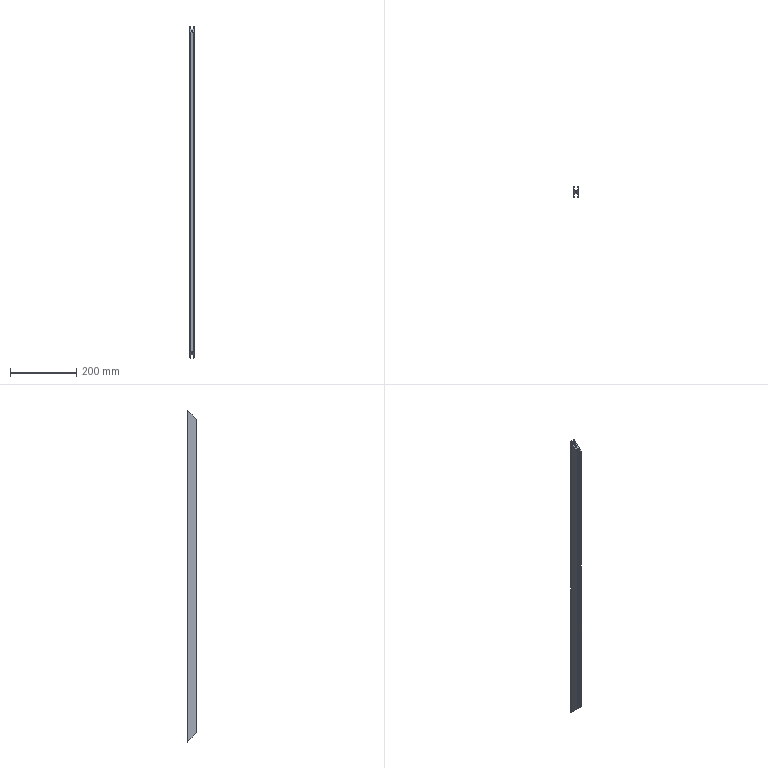Part | STEP file | OB1530-1000 | 1 solid | 36 faces | box 15 x 30 x 1000 mm | volume 237102 mm3 | plane 30 | cylinder 6 | commonest cylinder face diameters 3 x4 5 x2
STEP:
#1=CARTESIAN_POINT('',(2.5,0.,985.));
#2=VERTEX_POINT('',#1);
#3=CARTESIAN_POINT('',(-2.5,0.,985.));
#4=VERTEX_POINT('',#3);
#5=CARTESIAN_POINT('',(2.5,0.,985.));
#6=CARTESIAN_POINT('',(2.5,-5.,980.));
#7=CARTESIAN_POINT('',(-2.5,-5.,980.));
#8=CARTESIAN_POINT('',(-2.5,0.,985.));
#9=(BOUNDED_CURVE()B_SPLINE_CURVE(3,(#5,#6,#7,#8),.UNSPECIFIED.,.F.,.F.)B_SPLINE_CURVE_WITH_KNOTS((4,4),(4.712,7.854),.UNSPECIFIED.)CURVE()GEOMETRIC_REPRESENTATION_ITEM()RATIONAL_B_SPLINE_CURVE((1.,0.3333,0.3333,1.))REPRESENTATION_ITEM(''));
#10=EDGE_CURVE('',#2,#4,#9,.T.);
#11=ORIENTED_EDGE('',*,*,#10,.F.);
#12=CARTESIAN_POINT('',(2.5,0.,15.));
#13=VERTEX_POINT('',#12);
#14=CARTESIAN_POINT('',(2.5,0.,1000.));
#15=DIRECTION('',(0.,0.,-1.));
#16=VECTOR('',#15,1000.);
#17=LINE('',#14,#16);
#18=EDGE_CURVE('',#2,#13,#17,.T.);
#19=ORIENTED_EDGE('',*,*,#18,.T.);
#20=CARTESIAN_POINT('',(-2.5,0.,15.));
#21=VERTEX_POINT('',#20);
#22=CARTESIAN_POINT('',(-2.5,0.,15.));
#23=CARTESIAN_POINT('',(-2.5,-5.,20.));
#24=CARTESIAN_POINT('',(2.5,-5.,20.));
#25=CARTESIAN_POINT('',(2.5,0.,15.));
#26=(BOUNDED_CURVE()B_SPLINE_CURVE(3,(#22,#23,#24,#25),.UNSPECIFIED.,.F.,.F.)B_SPLINE_CURVE_WITH_KNOTS((4,4),(1.571,4.712),.UNSPECIFIED.)CURVE()GEOMETRIC_REPRESENTATION_ITEM()RATIONAL_B_SPLINE_CURVE((1.,0.3333,0.3333,1.))REPRESENTATION_ITEM(''));
#27=EDGE_CURVE('',#21,#13,#26,.T.);
#28=ORIENTED_EDGE('',*,*,#27,.F.);
#29=CARTESIAN_POINT('',(-2.5,0.,1000.));
#30=DIRECTION('',(0.,0.,-1.));
#31=VECTOR('',#30,1000.);
#32=LINE('',#29,#31);
#33=EDGE_CURVE('',#4,#21,#32,.T.);
#34=ORIENTED_EDGE('',*,*,#33,.F.);
#35=EDGE_LOOP('',(#11,#19,#28,#34));
#36=FACE_OUTER_BOUND('',#35,.T.);
#37=CARTESIAN_POINT('',(0.,0.,1000.));
#38=DIRECTION('',(0.,0.,-1.));
#39=DIRECTION('',(-1.,0.,0.));
#40=AXIS2_PLACEMENT_3D('',#37,#38,#39);
#41=CYLINDRICAL_SURFACE('',#40,2.5);
#42=ADVANCED_FACE('',(#36),#41,.F.);
#43=CARTESIAN_POINT('',(6.,15.,1000.));
#44=VERTEX_POINT('',#43);
#45=CARTESIAN_POINT('',(6.,15.,0.));
#46=VERTEX_POINT('',#45);
#47=CARTESIAN_POINT('',(6.,15.,1000.));
#48=DIRECTION('',(0.,0.,-1.));
#49=VECTOR('',#48,1000.);
#50=LINE('',#47,#49);
#51=EDGE_CURVE('',#44,#46,#50,.T.);
#52=ORIENTED_EDGE('',*,*,#51,.F.);
#53=CARTESIAN_POINT('',(7.5,13.5,998.5));
#54=VERTEX_POINT('',#53);
#55=CARTESIAN_POINT('',(6.,15.,1000.));
#56=CARTESIAN_POINT('',(6.879,15.,1000.));
#57=CARTESIAN_POINT('',(7.5,14.379,999.379));
#58=CARTESIAN_POINT('',(7.5,13.5,998.5));
#59=(BOUNDED_CURVE()B_SPLINE_CURVE(3,(#55,#56,#57,#58),.UNSPECIFIED.,.F.,.F.)B_SPLINE_CURVE_WITH_KNOTS((4,4),(3.142,4.712),.UNSPECIFIED.)CURVE()GEOMETRIC_REPRESENTATION_ITEM()RATIONAL_B_SPLINE_CURVE((1.,0.8047,0.8047,1.))REPRESENTATION_ITEM(''));
#60=EDGE_CURVE('',#44,#54,#59,.T.);
#61=ORIENTED_EDGE('',*,*,#60,.T.);
#62=CARTESIAN_POINT('',(7.5,13.5,1.5));
#63=VERTEX_POINT('',#62);
#64=CARTESIAN_POINT('',(7.5,13.5,1000.));
#65=DIRECTION('',(0.,0.,-1.));
#66=VECTOR('',#65,1000.);
#67=LINE('',#64,#66);
#68=EDGE_CURVE('',#54,#63,#67,.T.);
#69=ORIENTED_EDGE('',*,*,#68,.T.);
#70=CARTESIAN_POINT('',(7.5,13.5,1.5));
#71=CARTESIAN_POINT('',(7.5,14.379,0.6213));
#72=CARTESIAN_POINT('',(6.879,15.,0.));
#73=CARTESIAN_POINT('',(6.,15.,0.));
#74=(BOUNDED_CURVE()B_SPLINE_CURVE(3,(#70,#71,#72,#73),.UNSPECIFIED.,.F.,.T.)B_SPLINE_CURVE_WITH_KNOTS((4,4),(4.712,6.283),.UNSPECIFIED.)CURVE()GEOMETRIC_REPRESENTATION_ITEM()RATIONAL_B_SPLINE_CURVE((1.,0.8047,0.8047,1.))REPRESENTATION_ITEM(''));
#75=EDGE_CURVE('',#63,#46,#74,.T.);
#76=ORIENTED_EDGE('',*,*,#75,.T.);
#77=EDGE_LOOP('',(#52,#61,#69,#76));
#78=FACE_OUTER_BOUND('',#77,.T.);
#79=CARTESIAN_POINT('',(6.,13.5,1000.));
#80=DIRECTION('',(0.,0.,-1.));
#81=DIRECTION('',(-1.,0.,0.));
#82=AXIS2_PLACEMENT_3D('',#79,#80,#81);
#83=CYLINDRICAL_SURFACE('',#82,1.5);
#84=ADVANCED_FACE('',(#78),#83,.T.);
#85=CARTESIAN_POINT('',(3.25,15.,0.));
#86=VERTEX_POINT('',#85);
#87=CARTESIAN_POINT('',(6.,15.,0.));
#88=DIRECTION('',(-1.,0.,0.));
#89=VECTOR('',#88,1000.);
#90=LINE('',#87,#89);
#91=EDGE_CURVE('',#46,#86,#90,.T.);
#92=ORIENTED_EDGE('',*,*,#91,.T.);
#93=CARTESIAN_POINT('',(3.25,15.,1000.));
#94=VERTEX_POINT('',#93);
#95=CARTESIAN_POINT('',(3.25,15.,1000.));
#96=DIRECTION('',(0.,0.,-1.));
#97=VECTOR('',#96,1000.);
#98=LINE('',#95,#97);
#99=EDGE_CURVE('',#94,#86,#98,.T.);
#100=ORIENTED_EDGE('',*,*,#99,.F.);
#101=CARTESIAN_POINT('',(6.,15.,1000.));
#102=DIRECTION('',(-1.,0.,0.));
#103=VECTOR('',#102,1000.);
#104=LINE('',#101,#103);
#105=EDGE_CURVE('',#44,#94,#104,.T.);
#106=ORIENTED_EDGE('',*,*,#105,.F.);
#107=ORIENTED_EDGE('',*,*,#51,.T.);
#108=EDGE_LOOP('',(#92,#100,#106,#107));
#109=FACE_OUTER_BOUND('',#108,.T.);
#110=CARTESIAN_POINT('',(6.,15.,1000.));
#111=DIRECTION('',(0.,-1.,0.));
#112=DIRECTION('',(0.,0.,-1.));
#113=AXIS2_PLACEMENT_3D('',#110,#111,#112);
#114=PLANE('',#113);
#115=ADVANCED_FACE('',(#109),#114,.F.);
#116=CARTESIAN_POINT('',(3.25,13.,998.));
#117=VERTEX_POINT('',#116);
#118=CARTESIAN_POINT('',(3.25,13.,2.));
#119=VERTEX_POINT('',#118);
#120=CARTESIAN_POINT('',(3.25,13.,1000.));
#121=DIRECTION('',(0.,0.,-1.));
#122=VECTOR('',#121,1000.);
#123=LINE('',#120,#122);
#124=EDGE_CURVE('',#117,#119,#123,.T.);
#125=ORIENTED_EDGE('',*,*,#124,.F.);
#126=CARTESIAN_POINT('',(3.25,15.,1000.));
#127=DIRECTION('',(0.,0.7071,0.7071));
#128=VECTOR('',#127,1000.);
#129=LINE('',#126,#128);
#130=EDGE_CURVE('',#117,#94,#129,.T.);
#131=ORIENTED_EDGE('',*,*,#130,.T.);
#132=ORIENTED_EDGE('',*,*,#99,.T.);
#133=CARTESIAN_POINT('',(3.25,-485.,500.));
#134=DIRECTION('',(0.,-0.7071,0.7071));
#135=VECTOR('',#134,1000.);
#136=LINE('',#133,#135);
#137=EDGE_CURVE('',#86,#119,#136,.T.);
#138=ORIENTED_EDGE('',*,*,#137,.T.);
#139=EDGE_LOOP('',(#125,#131,#132,#138));
#140=FACE_OUTER_BOUND('',#139,.T.);
#141=CARTESIAN_POINT('',(3.25,15.,1000.));
#142=DIRECTION('',(1.,0.,0.));
#143=DIRECTION('',(0.,0.,-1.));
#144=AXIS2_PLACEMENT_3D('',#141,#142,#143);
#145=PLANE('',#144);
#146=ADVANCED_FACE('',(#140),#145,.F.);
#147=CARTESIAN_POINT('',(5.5,13.,998.));
#148=VERTEX_POINT('',#147);
#149=CARTESIAN_POINT('',(5.5,13.,2.));
#150=VERTEX_POINT('',#149);
#151=CARTESIAN_POINT('',(5.5,13.,1000.));
#152=DIRECTION('',(0.,0.,-1.));
#153=VECTOR('',#152,1000.);
#154=LINE('',#151,#153);
#155=EDGE_CURVE('',#148,#150,#154,.T.);
#156=ORIENTED_EDGE('',*,*,#155,.F.);
#157=CARTESIAN_POINT('',(3.25,13.,998.));
#158=DIRECTION('',(-1.,0.,0.));
#159=VECTOR('',#158,1000.);
#160=LINE('',#157,#159);
#161=EDGE_CURVE('',#148,#117,#160,.T.);
#162=ORIENTED_EDGE('',*,*,#161,.T.);
#163=ORIENTED_EDGE('',*,*,#124,.T.);
#164=CARTESIAN_POINT('',(3.25,13.,2.));
#165=DIRECTION('',(1.,0.,0.));
#166=VECTOR('',#165,1000.);
#167=LINE('',#164,#166);
#168=EDGE_CURVE('',#119,#150,#167,.T.);
#169=ORIENTED_EDGE('',*,*,#168,.T.);
#170=EDGE_LOOP('',(#156,#162,#163,#169));
#171=FACE_OUTER_BOUND('',#170,.T.);
#172=CARTESIAN_POINT('',(3.25,13.,1000.));
#173=DIRECTION('',(0.,1.,0.));
#174=DIRECTION('',(0.,0.,1.));
#175=AXIS2_PLACEMENT_3D('',#172,#173,#174);
#176=PLANE('',#175);
#177=ADVANCED_FACE('',(#171),#176,.F.);
#178=CARTESIAN_POINT('',(5.5,7.,992.));
#179=VERTEX_POINT('',#178);
#180=CARTESIAN_POINT('',(5.5,7.,8.));
#181=VERTEX_POINT('',#180);
#182=CARTESIAN_POINT('',(5.5,7.,1000.));
#183=DIRECTION('',(0.,0.,-1.));
#184=VECTOR('',#183,1000.);
#185=LINE('',#182,#184);
#186=EDGE_CURVE('',#179,#181,#185,.T.);
#187=ORIENTED_EDGE('',*,*,#186,.F.);
#188=CARTESIAN_POINT('',(5.5,14.,999.));
#189=DIRECTION('',(0.,0.7071,0.7071));
#190=VECTOR('',#189,1000.);
#191=LINE('',#188,#190);
#192=EDGE_CURVE('',#179,#148,#191,.T.);
#193=ORIENTED_EDGE('',*,*,#192,.T.);
#194=ORIENTED_EDGE('',*,*,#155,.T.);
#195=CARTESIAN_POINT('',(5.5,-486.,501.));
#196=DIRECTION('',(0.,-0.7071,0.7071));
#197=VECTOR('',#196,1000.);
#198=LINE('',#195,#197);
#199=EDGE_CURVE('',#150,#181,#198,.T.);
#200=ORIENTED_EDGE('',*,*,#199,.T.);
#201=EDGE_LOOP('',(#187,#193,#194,#200));
#202=FACE_OUTER_BOUND('',#201,.T.);
#203=CARTESIAN_POINT('',(5.5,13.,1000.));
#204=DIRECTION('',(1.,0.,0.));
#205=DIRECTION('',(0.,1.,0.));
#206=AXIS2_PLACEMENT_3D('',#203,#204,#205);
#207=PLANE('',#206);
#208=ADVANCED_FACE('',(#202),#207,.F.);
#209=CARTESIAN_POINT('',(3.25,7.,992.));
#210=VERTEX_POINT('',#209);
#211=CARTESIAN_POINT('',(3.25,7.,8.));
#212=VERTEX_POINT('',#211);
#213=CARTESIAN_POINT('',(3.25,7.,1000.));
#214=DIRECTION('',(0.,0.,-1.));
#215=VECTOR('',#214,1000.);
#216=LINE('',#213,#215);
#217=EDGE_CURVE('',#210,#212,#216,.T.);
#218=ORIENTED_EDGE('',*,*,#217,.F.);
#219=CARTESIAN_POINT('',(5.5,7.,992.));
#220=DIRECTION('',(1.,0.,0.));
#221=VECTOR('',#220,1000.);
#222=LINE('',#219,#221);
#223=EDGE_CURVE('',#210,#179,#222,.T.);
#224=ORIENTED_EDGE('',*,*,#223,.T.);
#225=ORIENTED_EDGE('',*,*,#186,.T.);
#226=CARTESIAN_POINT('',(5.5,7.,8.));
#227=DIRECTION('',(-1.,0.,0.));
#228=VECTOR('',#227,1000.);
#229=LINE('',#226,#228);
#230=EDGE_CURVE('',#181,#212,#229,.T.);
#231=ORIENTED_EDGE('',*,*,#230,.T.);
#232=EDGE_LOOP('',(#218,#224,#225,#231));
#233=FACE_OUTER_BOUND('',#232,.T.);
#234=CARTESIAN_POINT('',(5.5,7.,1000.));
#235=DIRECTION('',(0.,-1.,0.));
#236=DIRECTION('',(1.,0.,0.));
#237=AXIS2_PLACEMENT_3D('',#234,#235,#236);
#238=PLANE('',#237);
#239=ADVANCED_FACE('',(#233),#238,.F.);
#240=CARTESIAN_POINT('',(3.25,5.,990.));
#241=VERTEX_POINT('',#240);
#242=CARTESIAN_POINT('',(3.25,5.,10.));
#243=VERTEX_POINT('',#242);
#244=CARTESIAN_POINT('',(3.25,5.,1000.));
#245=DIRECTION('',(0.,0.,-1.));
#246=VECTOR('',#245,1000.);
#247=LINE('',#244,#246);
#248=EDGE_CURVE('',#241,#243,#247,.T.);
#249=ORIENTED_EDGE('',*,*,#248,.F.);
#250=CARTESIAN_POINT('',(3.25,11.,996.));
#251=DIRECTION('',(0.,0.7071,0.7071));
#252=VECTOR('',#251,1000.);
#253=LINE('',#250,#252);
#254=EDGE_CURVE('',#241,#210,#253,.T.);
#255=ORIENTED_EDGE('',*,*,#254,.T.);
#256=ORIENTED_EDGE('',*,*,#217,.T.);
#257=CARTESIAN_POINT('',(3.25,-489.,504.));
#258=DIRECTION('',(0.,-0.7071,0.7071));
#259=VECTOR('',#258,1000.);
#260=LINE('',#257,#259);
#261=EDGE_CURVE('',#212,#243,#260,.T.);
#262=ORIENTED_EDGE('',*,*,#261,.T.);
#263=EDGE_LOOP('',(#249,#255,#256,#262));
#264=FACE_OUTER_BOUND('',#263,.T.);
#265=CARTESIAN_POINT('',(3.25,7.,1000.));
#266=DIRECTION('',(1.,0.,0.));
#267=DIRECTION('',(0.,1.,0.));
#268=AXIS2_PLACEMENT_3D('',#265,#266,#267);
#269=PLANE('',#268);
#270=ADVANCED_FACE('',(#264),#269,.F.);
#271=CARTESIAN_POINT('',(-3.25,5.,990.));
#272=VERTEX_POINT('',#271);
#273=CARTESIAN_POINT('',(-3.25,5.,10.));
#274=VERTEX_POINT('',#273);
#275=CARTESIAN_POINT('',(-3.25,5.,1000.));
#276=DIRECTION('',(0.,0.,-1.));
#277=VECTOR('',#276,1000.);
#278=LINE('',#275,#277);
#279=EDGE_CURVE('',#272,#274,#278,.T.);
#280=ORIENTED_EDGE('',*,*,#279,.F.);
#281=CARTESIAN_POINT('',(3.25,5.,990.));
#282=DIRECTION('',(1.,0.,0.));
#283=VECTOR('',#282,1000.);
#284=LINE('',#281,#283);
#285=EDGE_CURVE('',#272,#241,#284,.T.);
#286=ORIENTED_EDGE('',*,*,#285,.T.);
#287=ORIENTED_EDGE('',*,*,#248,.T.);
#288=CARTESIAN_POINT('',(3.25,5.,10.));
#289=DIRECTION('',(-1.,0.,0.));
#290=VECTOR('',#289,1000.);
#291=LINE('',#288,#290);
#292=EDGE_CURVE('',#243,#274,#291,.T.);
#293=ORIENTED_EDGE('',*,*,#292,.T.);
#294=EDGE_LOOP('',(#280,#286,#287,#293));
#295=FACE_OUTER_BOUND('',#294,.T.);
#296=CARTESIAN_POINT('',(3.25,5.,1000.));
#297=DIRECTION('',(0.,-1.,0.));
#298=DIRECTION('',(0.,0.,-1.));
#299=AXIS2_PLACEMENT_3D('',#296,#297,#298);
#300=PLANE('',#299);
#301=ADVANCED_FACE('',(#295),#300,.F.);
#302=CARTESIAN_POINT('',(-3.25,7.,992.));
#303=VERTEX_POINT('',#302);
#304=CARTESIAN_POINT('',(-3.25,7.,8.));
#305=VERTEX_POINT('',#304);
#306=CARTESIAN_POINT('',(-3.25,7.,1000.));
#307=DIRECTION('',(0.,0.,-1.));
#308=VECTOR('',#307,1000.);
#309=LINE('',#306,#308);
#310=EDGE_CURVE('',#303,#305,#309,.T.);
#311=ORIENTED_EDGE('',*,*,#310,.F.);
#312=CARTESIAN_POINT('',(-3.25,11.,996.));
#313=DIRECTION('',(0.,-0.7071,-0.7071));
#314=VECTOR('',#313,1000.);
#315=LINE('',#312,#314);
#316=EDGE_CURVE('',#303,#272,#315,.T.);
#317=ORIENTED_EDGE('',*,*,#316,.T.);
#318=ORIENTED_EDGE('',*,*,#279,.T.);
#319=CARTESIAN_POINT('',(-3.25,-489.,504.));
#320=DIRECTION('',(0.,0.7071,-0.7071));
#321=VECTOR('',#320,1000.);
#322=LINE('',#319,#321);
#323=EDGE_CURVE('',#274,#305,#322,.T.);
#324=ORIENTED_EDGE('',*,*,#323,.T.);
#325=EDGE_LOOP('',(#311,#317,#318,#324));
#326=FACE_OUTER_BOUND('',#325,.T.);
#327=CARTESIAN_POINT('',(-3.25,7.,1000.));
#328=DIRECTION('',(-1.,0.,0.));
#329=DIRECTION('',(0.,-1.,0.));
#330=AXIS2_PLACEMENT_3D('',#327,#328,#329);
#331=PLANE('',#330);
#332=ADVANCED_FACE('',(#326),#331,.F.);
#333=CARTESIAN_POINT('',(-5.5,7.,992.));
#334=VERTEX_POINT('',#333);
#335=CARTESIAN_POINT('',(-5.5,7.,8.));
#336=VERTEX_POINT('',#335);
#337=CARTESIAN_POINT('',(-5.5,7.,1000.));
#338=DIRECTION('',(0.,0.,-1.));
#339=VECTOR('',#338,1000.);
#340=LINE('',#337,#339);
#341=EDGE_CURVE('',#334,#336,#340,.T.);
#342=ORIENTED_EDGE('',*,*,#341,.F.);
#343=CARTESIAN_POINT('',(-5.5,7.,992.));
#344=DIRECTION('',(1.,0.,0.));
#345=VECTOR('',#344,1000.);
#346=LINE('',#343,#345);
#347=EDGE_CURVE('',#334,#303,#346,.T.);
#348=ORIENTED_EDGE('',*,*,#347,.T.);
#349=ORIENTED_EDGE('',*,*,#310,.T.);
#350=CARTESIAN_POINT('',(-5.5,7.,8.));
#351=DIRECTION('',(-1.,0.,0.));
#352=VECTOR('',#351,1000.);
#353=LINE('',#350,#352);
#354=EDGE_CURVE('',#305,#336,#353,.T.);
#355=ORIENTED_EDGE('',*,*,#354,.T.);
#356=EDGE_LOOP('',(#342,#348,#349,#355));
#357=FACE_OUTER_BOUND('',#356,.T.);
#358=CARTESIAN_POINT('',(-5.5,7.,1000.));
#359=DIRECTION('',(0.,-1.,0.));
#360=DIRECTION('',(1.,0.,0.));
#361=AXIS2_PLACEMENT_3D('',#358,#359,#360);
#362=PLANE('',#361);
#363=ADVANCED_FACE('',(#357),#362,.F.);
#364=CARTESIAN_POINT('',(-5.5,13.,998.));
#365=VERTEX_POINT('',#364);
#366=CARTESIAN_POINT('',(-5.5,13.,2.));
#367=VERTEX_POINT('',#366);
#368=CARTESIAN_POINT('',(-5.5,13.,1000.));
#369=DIRECTION('',(0.,0.,-1.));
#370=VECTOR('',#369,1000.);
#371=LINE('',#368,#370);
#372=EDGE_CURVE('',#365,#367,#371,.T.);
#373=ORIENTED_EDGE('',*,*,#372,.F.);
#374=CARTESIAN_POINT('',(-5.5,14.,999.));
#375=DIRECTION('',(0.,-0.7071,-0.7071));
#376=VECTOR('',#375,1000.);
#377=LINE('',#374,#376);
#378=EDGE_CURVE('',#365,#334,#377,.T.);
#379=ORIENTED_EDGE('',*,*,#378,.T.);
#380=ORIENTED_EDGE('',*,*,#341,.T.);
#381=CARTESIAN_POINT('',(-5.5,-486.,501.));
#382=DIRECTION('',(0.,0.7071,-0.7071));
#383=VECTOR('',#382,1000.);
#384=LINE('',#381,#383);
#385=EDGE_CURVE('',#336,#367,#384,.T.);
#386=ORIENTED_EDGE('',*,*,#385,.T.);
#387=EDGE_LOOP('',(#373,#379,#380,#386));
#388=FACE_OUTER_BOUND('',#387,.T.);
#389=CARTESIAN_POINT('',(-5.5,13.,1000.));
#390=DIRECTION('',(-1.,0.,0.));
#391=DIRECTION('',(0.,-1.,0.));
#392=AXIS2_PLACEMENT_3D('',#389,#390,#391);
#393=PLANE('',#392);
#394=ADVANCED_FACE('',(#388),#393,.F.);
#395=CARTESIAN_POINT('',(-3.25,13.,998.));
#396=VERTEX_POINT('',#395);
#397=CARTESIAN_POINT('',(-3.25,13.,2.));
#398=VERTEX_POINT('',#397);
#399=CARTESIAN_POINT('',(-3.25,13.,1000.));
#400=DIRECTION('',(0.,0.,-1.));
#401=VECTOR('',#400,1000.);
#402=LINE('',#399,#401);
#403=EDGE_CURVE('',#396,#398,#402,.T.);
#404=ORIENTED_EDGE('',*,*,#403,.F.);
#405=CARTESIAN_POINT('',(-3.25,13.,998.));
#406=DIRECTION('',(-1.,0.,0.));
#407=VECTOR('',#406,1000.);
#408=LINE('',#405,#407);
#409=EDGE_CURVE('',#396,#365,#408,.T.);
#410=ORIENTED_EDGE('',*,*,#409,.T.);
#411=ORIENTED_EDGE('',*,*,#372,.T.);
#412=CARTESIAN_POINT('',(-3.25,13.,2.));
#413=DIRECTION('',(1.,0.,0.));
#414=VECTOR('',#413,1000.);
#415=LINE('',#412,#414);
#416=EDGE_CURVE('',#367,#398,#415,.T.);
#417=ORIENTED_EDGE('',*,*,#416,.T.);
#418=EDGE_LOOP('',(#404,#410,#411,#417));
#419=FACE_OUTER_BOUND('',#418,.T.);
#420=CARTESIAN_POINT('',(-3.25,13.,1000.));
#421=DIRECTION('',(0.,1.,0.));
#422=DIRECTION('',(0.,0.,1.));
#423=AXIS2_PLACEMENT_3D('',#420,#421,#422);
#424=PLANE('',#423);
#425=ADVANCED_FACE('',(#419),#424,.F.);
#426=CARTESIAN_POINT('',(-3.25,15.,1000.));
#427=VERTEX_POINT('',#426);
#428=CARTESIAN_POINT('',(-3.25,15.,0.));
#429=VERTEX_POINT('',#428);
#430=CARTESIAN_POINT('',(-3.25,15.,1000.));
#431=DIRECTION('',(0.,0.,-1.));
#432=VECTOR('',#431,1000.);
#433=LINE('',#430,#432);
#434=EDGE_CURVE('',#427,#429,#433,.T.);
#435=ORIENTED_EDGE('',*,*,#434,.F.);
#436=CARTESIAN_POINT('',(-3.25,15.,1000.));
#437=DIRECTION('',(0.,-0.7071,-0.7071));
#438=VECTOR('',#437,1000.);
#439=LINE('',#436,#438);
#440=EDGE_CURVE('',#427,#396,#439,.T.);
#441=ORIENTED_EDGE('',*,*,#440,.T.);
#442=ORIENTED_EDGE('',*,*,#403,.T.);
#443=CARTESIAN_POINT('',(-3.25,-485.,500.));
#444=DIRECTION('',(0.,0.7071,-0.7071));
#445=VECTOR('',#444,1000.);
#446=LINE('',#443,#445);
#447=EDGE_CURVE('',#398,#429,#446,.T.);
#448=ORIENTED_EDGE('',*,*,#447,.T.);
#449=EDGE_LOOP('',(#435,#441,#442,#448));
#450=FACE_OUTER_BOUND('',#449,.T.);
#451=CARTESIAN_POINT('',(-3.25,15.,1000.));
#452=DIRECTION('',(-1.,0.,0.));
#453=DIRECTION('',(0.,0.,1.));
#454=AXIS2_PLACEMENT_3D('',#451,#452,#453);
#455=PLANE('',#454);
#456=ADVANCED_FACE('',(#450),#455,.F.);
#457=CARTESIAN_POINT('',(-6.,15.,0.));
#458=VERTEX_POINT('',#457);
#459=CARTESIAN_POINT('',(-6.,15.,0.));
#460=DIRECTION('',(-1.,0.,0.));
#461=VECTOR('',#460,1000.);
#462=LINE('',#459,#461);
#463=EDGE_CURVE('',#429,#458,#462,.T.);
#464=ORIENTED_EDGE('',*,*,#463,.T.);
#465=CARTESIAN_POINT('',(-6.,15.,1000.));
#466=VERTEX_POINT('',#465);
#467=CARTESIAN_POINT('',(-6.,15.,1000.));
#468=DIRECTION('',(0.,0.,-1.));
#469=VECTOR('',#468,1000.);
#470=LINE('',#467,#469);
#471=EDGE_CURVE('',#466,#458,#470,.T.);
#472=ORIENTED_EDGE('',*,*,#471,.F.);
#473=CARTESIAN_POINT('',(-6.,15.,1000.));
#474=DIRECTION('',(-1.,0.,0.));
#475=VECTOR('',#474,1000.);
#476=LINE('',#473,#475);
#477=EDGE_CURVE('',#427,#466,#476,.T.);
#478=ORIENTED_EDGE('',*,*,#477,.F.);
#479=ORIENTED_EDGE('',*,*,#434,.T.);
#480=EDGE_LOOP('',(#464,#472,#478,#479));
#481=FACE_OUTER_BOUND('',#480,.T.);
#482=CARTESIAN_POINT('',(-6.,15.,1000.));
#483=DIRECTION('',(0.,-1.,0.));
#484=DIRECTION('',(0.,0.,-1.));
#485=AXIS2_PLACEMENT_3D('',#482,#483,#484);
#486=PLANE('',#485);
#487=ADVANCED_FACE('',(#481),#486,.F.);
#488=CARTESIAN_POINT('',(-7.5,13.5,998.5));
#489=VERTEX_POINT('',#488);
#490=CARTESIAN_POINT('',(-7.5,13.5,1.5));
#491=VERTEX_POINT('',#490);
#492=CARTESIAN_POINT('',(-7.5,13.5,1000.));
#493=DIRECTION('',(0.,0.,-1.));
#494=VECTOR('',#493,1000.);
#495=LINE('',#492,#494);
#496=EDGE_CURVE('',#489,#491,#495,.T.);
#497=ORIENTED_EDGE('',*,*,#496,.F.);
#498=CARTESIAN_POINT('',(-7.5,13.5,998.5));
#499=CARTESIAN_POINT('',(-7.5,14.379,999.379));
#500=CARTESIAN_POINT('',(-6.879,15.,1000.));
#501=CARTESIAN_POINT('',(-6.,15.,1000.));
#502=(BOUNDED_CURVE()B_SPLINE_CURVE(3,(#498,#499,#500,#501),.UNSPECIFIED.,.F.,.F.)B_SPLINE_CURVE_WITH_KNOTS((4,4),(1.571,3.142),.UNSPECIFIED.)CURVE()GEOMETRIC_REPRESENTATION_ITEM()RATIONAL_B_SPLINE_CURVE((1.,0.8047,0.8047,1.))REPRESENTATION_ITEM(''));
#503=EDGE_CURVE('',#489,#466,#502,.T.);
#504=ORIENTED_EDGE('',*,*,#503,.T.);
#505=ORIENTED_EDGE('',*,*,#471,.T.);
#506=CARTESIAN_POINT('',(-6.,15.,0.));
#507=CARTESIAN_POINT('',(-6.879,15.,0.));
#508=CARTESIAN_POINT('',(-7.5,14.379,0.6213));
#509=CARTESIAN_POINT('',(-7.5,13.5,1.5));
#510=(BOUNDED_CURVE()B_SPLINE_CURVE(3,(#506,#507,#508,#509),.UNSPECIFIED.,.F.,.F.)B_SPLINE_CURVE_WITH_KNOTS((4,4),(0.,1.571),.UNSPECIFIED.)CURVE()GEOMETRIC_REPRESENTATION_ITEM()RATIONAL_B_SPLINE_CURVE((1.,0.8047,0.8047,1.))REPRESENTATION_ITEM(''));
#511=EDGE_CURVE('',#458,#491,#510,.T.);
#512=ORIENTED_EDGE('',*,*,#511,.T.);
#513=EDGE_LOOP('',(#497,#504,#505,#512));
#514=FACE_OUTER_BOUND('',#513,.T.);
#515=CARTESIAN_POINT('',(-6.,13.5,1000.));
#516=DIRECTION('',(0.,0.,-1.));
#517=DIRECTION('',(-1.,0.,0.));
#518=AXIS2_PLACEMENT_3D('',#515,#516,#517);
#519=CYLINDRICAL_SURFACE('',#518,1.5);
#520=ADVANCED_FACE('',(#514),#519,.T.);
#521=CARTESIAN_POINT('',(-7.5,-13.5,971.5));
#522=VERTEX_POINT('',#521);
#523=CARTESIAN_POINT('',(-7.5,-13.5,28.5));
#524=VERTEX_POINT('',#523);
#525=CARTESIAN_POINT('',(-7.5,-13.5,1000.));
#526=DIRECTION('',(0.,0.,-1.));
#527=VECTOR('',#526,1000.);
#528=LINE('',#525,#527);
#529=EDGE_CURVE('',#522,#524,#528,.T.);
#530=ORIENTED_EDGE('',*,*,#529,.F.);
#531=CARTESIAN_POINT('',(-7.5,-15.,970.));
#532=DIRECTION('',(0.,-0.7071,-0.7071));
#533=VECTOR('',#532,1000.);
#534=LINE('',#531,#533);
#535=EDGE_CURVE('',#489,#522,#534,.T.);
#536=ORIENTED_EDGE('',*,*,#535,.F.);
#537=ORIENTED_EDGE('',*,*,#496,.T.);
#538=CARTESIAN_POINT('',(-7.5,15.,0.));
#539=DIRECTION('',(0.,0.7071,-0.7071));
#540=VECTOR('',#539,1000.);
#541=LINE('',#538,#540);
#542=EDGE_CURVE('',#524,#491,#541,.T.);
#543=ORIENTED_EDGE('',*,*,#542,.F.);
#544=EDGE_LOOP('',(#530,#536,#537,#543));
#545=FACE_OUTER_BOUND('',#544,.T.);
#546=CARTESIAN_POINT('',(-7.5,-13.5,1000.));
#547=DIRECTION('',(1.,0.,0.));
#548=DIRECTION('',(0.,0.,-1.));
#549=AXIS2_PLACEMENT_3D('',#546,#547,#548);
#550=PLANE('',#549);
#551=ADVANCED_FACE('',(#545),#550,.F.);
#552=CARTESIAN_POINT('',(-6.,-15.,970.));
#553=VERTEX_POINT('',#552);
#554=CARTESIAN_POINT('',(-6.,-15.,30.));
#555=VERTEX_POINT('',#554);
#556=CARTESIAN_POINT('',(-6.,-15.,1000.));
#557=DIRECTION('',(0.,0.,-1.));
#558=VECTOR('',#557,1000.);
#559=LINE('',#556,#558);
#560=EDGE_CURVE('',#553,#555,#559,.T.);
#561=ORIENTED_EDGE('',*,*,#560,.F.);
#562=CARTESIAN_POINT('',(-6.,-15.,970.));
#563=CARTESIAN_POINT('',(-6.879,-15.,970.));
#564=CARTESIAN_POINT('',(-7.5,-14.379,970.621));
#565=CARTESIAN_POINT('',(-7.5,-13.5,971.5));
#566=(BOUNDED_CURVE()B_SPLINE_CURVE(3,(#562,#563,#564,#565),.UNSPECIFIED.,.F.,.F.)B_SPLINE_CURVE_WITH_KNOTS((4,4),(0.,1.571),.UNSPECIFIED.)CURVE()GEOMETRIC_REPRESENTATION_ITEM()RATIONAL_B_SPLINE_CURVE((1.,0.8047,0.8047,1.))REPRESENTATION_ITEM(''));
#567=EDGE_CURVE('',#553,#522,#566,.T.);
#568=ORIENTED_EDGE('',*,*,#567,.T.);
#569=ORIENTED_EDGE('',*,*,#529,.T.);
#570=CARTESIAN_POINT('',(-7.5,-13.5,28.5));
#571=CARTESIAN_POINT('',(-7.5,-14.379,29.379));
#572=CARTESIAN_POINT('',(-6.879,-15.,30.));
#573=CARTESIAN_POINT('',(-6.,-15.,30.));
#574=(BOUNDED_CURVE()B_SPLINE_CURVE(3,(#570,#571,#572,#573),.UNSPECIFIED.,.F.,.T.)B_SPLINE_CURVE_WITH_KNOTS((4,4),(1.571,3.142),.UNSPECIFIED.)CURVE()GEOMETRIC_REPRESENTATION_ITEM()RATIONAL_B_SPLINE_CURVE((1.,0.8047,0.8047,1.))REPRESENTATION_ITEM(''));
#575=EDGE_CURVE('',#524,#555,#574,.T.);
#576=ORIENTED_EDGE('',*,*,#575,.T.);
#577=EDGE_LOOP('',(#561,#568,#569,#576));
#578=FACE_OUTER_BOUND('',#577,.T.);
#579=CARTESIAN_POINT('',(-6.,-13.5,1000.));
#580=DIRECTION('',(0.,0.,-1.));
#581=DIRECTION('',(-1.,0.,0.));
#582=AXIS2_PLACEMENT_3D('',#579,#580,#581);
#583=CYLINDRICAL_SURFACE('',#582,1.5);
#584=ADVANCED_FACE('',(#578),#583,.T.);
#585=CARTESIAN_POINT('',(-3.25,-15.,970.));
#586=VERTEX_POINT('',#585);
#587=CARTESIAN_POINT('',(-3.25,-15.,30.));
#588=VERTEX_POINT('',#587);
#589=CARTESIAN_POINT('',(-3.25,-15.,1000.));
#590=DIRECTION('',(0.,0.,-1.));
#591=VECTOR('',#590,1000.);
#592=LINE('',#589,#591);
#593=EDGE_CURVE('',#586,#588,#592,.T.);
#594=ORIENTED_EDGE('',*,*,#593,.F.);
#595=CARTESIAN_POINT('',(7.5,-15.,970.));
#596=DIRECTION('',(-1.,0.,0.));
#597=VECTOR('',#596,1000.);
#598=LINE('',#595,#597);
#599=EDGE_CURVE('',#586,#553,#598,.T.);
#600=ORIENTED_EDGE('',*,*,#599,.T.);
#601=ORIENTED_EDGE('',*,*,#560,.T.);
#602=CARTESIAN_POINT('',(7.5,-15.,30.));
#603=DIRECTION('',(-1.,0.,0.));
#604=VECTOR('',#603,1000.);
#605=LINE('',#602,#604);
#606=EDGE_CURVE('',#588,#555,#605,.T.);
#607=ORIENTED_EDGE('',*,*,#606,.F.);
#608=EDGE_LOOP('',(#594,#600,#601,#607));
#609=FACE_OUTER_BOUND('',#608,.T.);
#610=CARTESIAN_POINT('',(-6.,-15.,1000.));
#611=DIRECTION('',(0.,1.,0.));
#612=DIRECTION('',(0.,0.,1.));
#613=AXIS2_PLACEMENT_3D('',#610,#611,#612);
#614=PLANE('',#613);
#615=ADVANCED_FACE('',(#609),#614,.F.);
#616=CARTESIAN_POINT('',(-3.25,-13.,972.));
#617=VERTEX_POINT('',#616);
#618=CARTESIAN_POINT('',(-3.25,-13.,28.));
#619=VERTEX_POINT('',#618);
#620=CARTESIAN_POINT('',(-3.25,-13.,1000.));
#621=DIRECTION('',(0.,0.,-1.));
#622=VECTOR('',#621,1000.);
#623=LINE('',#620,#622);
#624=EDGE_CURVE('',#617,#619,#623,.T.);
#625=ORIENTED_EDGE('',*,*,#624,.F.);
#626=CARTESIAN_POINT('',(-3.25,0.,985.));
#627=DIRECTION('',(0.,-0.7071,-0.7071));
#628=VECTOR('',#627,1000.);
#629=LINE('',#626,#628);
#630=EDGE_CURVE('',#617,#586,#629,.T.);
#631=ORIENTED_EDGE('',*,*,#630,.T.);
#632=ORIENTED_EDGE('',*,*,#593,.T.);
#633=CARTESIAN_POINT('',(-3.25,-500.,515.));
#634=DIRECTION('',(0.,0.7071,-0.7071));
#635=VECTOR('',#634,1000.);
#636=LINE('',#633,#635);
#637=EDGE_CURVE('',#588,#619,#636,.T.);
#638=ORIENTED_EDGE('',*,*,#637,.T.);
#639=EDGE_LOOP('',(#625,#631,#632,#638));
#640=FACE_OUTER_BOUND('',#639,.T.);
#641=CARTESIAN_POINT('',(-3.25,-15.,1000.));
#642=DIRECTION('',(-1.,0.,0.));
#643=DIRECTION('',(0.,0.,1.));
#644=AXIS2_PLACEMENT_3D('',#641,#642,#643);
#645=PLANE('',#644);
#646=ADVANCED_FACE('',(#640),#645,.F.);
#647=CARTESIAN_POINT('',(-5.5,-13.,972.));
#648=VERTEX_POINT('',#647);
#649=CARTESIAN_POINT('',(-5.5,-13.,28.));
#650=VERTEX_POINT('',#649);
#651=CARTESIAN_POINT('',(-5.5,-13.,1000.));
#652=DIRECTION('',(0.,0.,-1.));
#653=VECTOR('',#652,1000.);
#654=LINE('',#651,#653);
#655=EDGE_CURVE('',#648,#650,#654,.T.);
#656=ORIENTED_EDGE('',*,*,#655,.F.);
#657=CARTESIAN_POINT('',(-3.25,-13.,972.));
#658=DIRECTION('',(1.,0.,0.));
#659=VECTOR('',#658,1000.);
#660=LINE('',#657,#659);
#661=EDGE_CURVE('',#648,#617,#660,.T.);
#662=ORIENTED_EDGE('',*,*,#661,.T.);
#663=ORIENTED_EDGE('',*,*,#624,.T.);
#664=CARTESIAN_POINT('',(-3.25,-13.,28.));
#665=DIRECTION('',(-1.,0.,0.));
#666=VECTOR('',#665,1000.);
#667=LINE('',#664,#666);
#668=EDGE_CURVE('',#619,#650,#667,.T.);
#669=ORIENTED_EDGE('',*,*,#668,.T.);
#670=EDGE_LOOP('',(#656,#662,#663,#669));
#671=FACE_OUTER_BOUND('',#670,.T.);
#672=CARTESIAN_POINT('',(-3.25,-13.,1000.));
#673=DIRECTION('',(0.,-1.,0.));
#674=DIRECTION('',(0.,0.,-1.));
#675=AXIS2_PLACEMENT_3D('',#672,#673,#674);
#676=PLANE('',#675);
#677=ADVANCED_FACE('',(#671),#676,.F.);
#678=CARTESIAN_POINT('',(-5.5,-7.,978.));
#679=VERTEX_POINT('',#678);
#680=CARTESIAN_POINT('',(-5.5,-7.,22.));
#681=VERTEX_POINT('',#680);
#682=CARTESIAN_POINT('',(-5.5,-7.,1000.));
#683=DIRECTION('',(0.,0.,-1.));
#684=VECTOR('',#683,1000.);
#685=LINE('',#682,#684);
#686=EDGE_CURVE('',#679,#681,#685,.T.);
#687=ORIENTED_EDGE('',*,*,#686,.F.);
#688=CARTESIAN_POINT('',(-5.5,1.,986.));
#689=DIRECTION('',(0.,-0.7071,-0.7071));
#690=VECTOR('',#689,1000.);
#691=LINE('',#688,#690);
#692=EDGE_CURVE('',#679,#648,#691,.T.);
#693=ORIENTED_EDGE('',*,*,#692,.T.);
#694=ORIENTED_EDGE('',*,*,#655,.T.);
#695=CARTESIAN_POINT('',(-5.5,-499.,514.));
#696=DIRECTION('',(0.,0.7071,-0.7071));
#697=VECTOR('',#696,1000.);
#698=LINE('',#695,#697);
#699=EDGE_CURVE('',#650,#681,#698,.T.);
#700=ORIENTED_EDGE('',*,*,#699,.T.);
#701=EDGE_LOOP('',(#687,#693,#694,#700));
#702=FACE_OUTER_BOUND('',#701,.T.);
#703=CARTESIAN_POINT('',(-5.5,-13.,1000.));
#704=DIRECTION('',(-1.,0.,0.));
#705=DIRECTION('',(0.,-1.,0.));
#706=AXIS2_PLACEMENT_3D('',#703,#704,#705);
#707=PLANE('',#706);
#708=ADVANCED_FACE('',(#702),#707,.F.);
#709=CARTESIAN_POINT('',(-3.25,-7.,978.));
#710=VERTEX_POINT('',#709);
#711=CARTESIAN_POINT('',(-3.25,-7.,22.));
#712=VERTEX_POINT('',#711);
#713=CARTESIAN_POINT('',(-3.25,-7.,1000.));
#714=DIRECTION('',(0.,0.,-1.));
#715=VECTOR('',#714,1000.);
#716=LINE('',#713,#715);
#717=EDGE_CURVE('',#710,#712,#716,.T.);
#718=ORIENTED_EDGE('',*,*,#717,.F.);
#719=CARTESIAN_POINT('',(-5.5,-7.,978.));
#720=DIRECTION('',(-1.,0.,0.));
#721=VECTOR('',#720,1000.);
#722=LINE('',#719,#721);
#723=EDGE_CURVE('',#710,#679,#722,.T.);
#724=ORIENTED_EDGE('',*,*,#723,.T.);
#725=ORIENTED_EDGE('',*,*,#686,.T.);
#726=CARTESIAN_POINT('',(-5.5,-7.,22.));
#727=DIRECTION('',(1.,0.,0.));
#728=VECTOR('',#727,1000.);
#729=LINE('',#726,#728);
#730=EDGE_CURVE('',#681,#712,#729,.T.);
#731=ORIENTED_EDGE('',*,*,#730,.T.);
#732=EDGE_LOOP('',(#718,#724,#725,#731));
#733=FACE_OUTER_BOUND('',#732,.T.);
#734=CARTESIAN_POINT('',(-5.5,-7.,1000.));
#735=DIRECTION('',(0.,1.,0.));
#736=DIRECTION('',(-1.,0.,0.));
#737=AXIS2_PLACEMENT_3D('',#734,#735,#736);
#738=PLANE('',#737);
#739=ADVANCED_FACE('',(#733),#738,.F.);
#740=CARTESIAN_POINT('',(-3.25,-5.,980.));
#741=VERTEX_POINT('',#740);
#742=CARTESIAN_POINT('',(-3.25,-5.,20.));
#743=VERTEX_POINT('',#742);
#744=CARTESIAN_POINT('',(-3.25,-5.,1000.));
#745=DIRECTION('',(0.,0.,-1.));
#746=VECTOR('',#745,1000.);
#747=LINE('',#744,#746);
#748=EDGE_CURVE('',#741,#743,#747,.T.);
#749=ORIENTED_EDGE('',*,*,#748,.F.);
#750=CARTESIAN_POINT('',(-3.25,4.,989.));
#751=DIRECTION('',(0.,-0.7071,-0.7071));
#752=VECTOR('',#751,1000.);
#753=LINE('',#750,#752);
#754=EDGE_CURVE('',#741,#710,#753,.T.);
#755=ORIENTED_EDGE('',*,*,#754,.T.);
#756=ORIENTED_EDGE('',*,*,#717,.T.);
#757=CARTESIAN_POINT('',(-3.25,-496.,511.));
#758=DIRECTION('',(0.,0.7071,-0.7071));
#759=VECTOR('',#758,1000.);
#760=LINE('',#757,#759);
#761=EDGE_CURVE('',#712,#743,#760,.T.);
#762=ORIENTED_EDGE('',*,*,#761,.T.);
#763=EDGE_LOOP('',(#749,#755,#756,#762));
#764=FACE_OUTER_BOUND('',#763,.T.);
#765=CARTESIAN_POINT('',(-3.25,-7.,1000.));
#766=DIRECTION('',(-1.,0.,0.));
#767=DIRECTION('',(0.,-1.,0.));
#768=AXIS2_PLACEMENT_3D('',#765,#766,#767);
#769=PLANE('',#768);
#770=ADVANCED_FACE('',(#764),#769,.F.);
#771=CARTESIAN_POINT('',(3.25,-5.,980.));
#772=VERTEX_POINT('',#771);
#773=CARTESIAN_POINT('',(3.25,-5.,20.));
#774=VERTEX_POINT('',#773);
#775=CARTESIAN_POINT('',(3.25,-5.,1000.));
#776=DIRECTION('',(0.,0.,-1.));
#777=VECTOR('',#776,1000.);
#778=LINE('',#775,#777);
#779=EDGE_CURVE('',#772,#774,#778,.T.);
#780=ORIENTED_EDGE('',*,*,#779,.F.);
#781=CARTESIAN_POINT('',(3.25,-5.,980.));
#782=DIRECTION('',(-1.,0.,0.));
#783=VECTOR('',#782,1000.);
#784=LINE('',#781,#783);
#785=EDGE_CURVE('',#772,#741,#784,.T.);
#786=ORIENTED_EDGE('',*,*,#785,.T.);
#787=ORIENTED_EDGE('',*,*,#748,.T.);
#788=CARTESIAN_POINT('',(3.25,-5.,20.));
#789=DIRECTION('',(1.,0.,0.));
#790=VECTOR('',#789,1000.);
#791=LINE('',#788,#790);
#792=EDGE_CURVE('',#743,#774,#791,.T.);
#793=ORIENTED_EDGE('',*,*,#792,.T.);
#794=EDGE_LOOP('',(#780,#786,#787,#793));
#795=FACE_OUTER_BOUND('',#794,.T.);
#796=CARTESIAN_POINT('',(3.25,-5.,1000.));
#797=DIRECTION('',(0.,1.,0.));
#798=DIRECTION('',(0.,0.,1.));
#799=AXIS2_PLACEMENT_3D('',#796,#797,#798);
#800=PLANE('',#799);
#801=ADVANCED_FACE('',(#795),#800,.F.);
#802=CARTESIAN_POINT('',(3.25,-7.,978.));
#803=VERTEX_POINT('',#802);
#804=CARTESIAN_POINT('',(3.25,-7.,22.));
#805=VERTEX_POINT('',#804);
#806=CARTESIAN_POINT('',(3.25,-7.,1000.));
#807=DIRECTION('',(0.,0.,-1.));
#808=VECTOR('',#807,1000.);
#809=LINE('',#806,#808);
#810=EDGE_CURVE('',#803,#805,#809,.T.);
#811=ORIENTED_EDGE('',*,*,#810,.F.);
#812=CARTESIAN_POINT('',(3.25,4.,989.));
#813=DIRECTION('',(0.,0.7071,0.7071));
#814=VECTOR('',#813,1000.);
#815=LINE('',#812,#814);
#816=EDGE_CURVE('',#803,#772,#815,.T.);
#817=ORIENTED_EDGE('',*,*,#816,.T.);
#818=ORIENTED_EDGE('',*,*,#779,.T.);
#819=CARTESIAN_POINT('',(3.25,-496.,511.));
#820=DIRECTION('',(0.,-0.7071,0.7071));
#821=VECTOR('',#820,1000.);
#822=LINE('',#819,#821);
#823=EDGE_CURVE('',#774,#805,#822,.T.);
#824=ORIENTED_EDGE('',*,*,#823,.T.);
#825=EDGE_LOOP('',(#811,#817,#818,#824));
#826=FACE_OUTER_BOUND('',#825,.T.);
#827=CARTESIAN_POINT('',(3.25,-7.,1000.));
#828=DIRECTION('',(1.,0.,0.));
#829=DIRECTION('',(0.,1.,0.));
#830=AXIS2_PLACEMENT_3D('',#827,#828,#829);
#831=PLANE('',#830);
#832=ADVANCED_FACE('',(#826),#831,.F.);
#833=CARTESIAN_POINT('',(5.5,-7.,978.));
#834=VERTEX_POINT('',#833);
#835=CARTESIAN_POINT('',(5.5,-7.,22.));
#836=VERTEX_POINT('',#835);
#837=CARTESIAN_POINT('',(5.5,-7.,1000.));
#838=DIRECTION('',(0.,0.,-1.));
#839=VECTOR('',#838,1000.);
#840=LINE('',#837,#839);
#841=EDGE_CURVE('',#834,#836,#840,.T.);
#842=ORIENTED_EDGE('',*,*,#841,.F.);
#843=CARTESIAN_POINT('',(5.5,-7.,978.));
#844=DIRECTION('',(-1.,0.,0.));
#845=VECTOR('',#844,1000.);
#846=LINE('',#843,#845);
#847=EDGE_CURVE('',#834,#803,#846,.T.);
#848=ORIENTED_EDGE('',*,*,#847,.T.);
#849=ORIENTED_EDGE('',*,*,#810,.T.);
#850=CARTESIAN_POINT('',(5.5,-7.,22.));
#851=DIRECTION('',(1.,0.,0.));
#852=VECTOR('',#851,1000.);
#853=LINE('',#850,#852);
#854=EDGE_CURVE('',#805,#836,#853,.T.);
#855=ORIENTED_EDGE('',*,*,#854,.T.);
#856=EDGE_LOOP('',(#842,#848,#849,#855));
#857=FACE_OUTER_BOUND('',#856,.T.);
#858=CARTESIAN_POINT('',(5.5,-7.,1000.));
#859=DIRECTION('',(0.,1.,0.));
#860=DIRECTION('',(-1.,0.,0.));
#861=AXIS2_PLACEMENT_3D('',#858,#859,#860);
#862=PLANE('',#861);
#863=ADVANCED_FACE('',(#857),#862,.F.);
#864=CARTESIAN_POINT('',(5.5,-13.,972.));
#865=VERTEX_POINT('',#864);
#866=CARTESIAN_POINT('',(5.5,-13.,28.));
#867=VERTEX_POINT('',#866);
#868=CARTESIAN_POINT('',(5.5,-13.,1000.));
#869=DIRECTION('',(0.,0.,-1.));
#870=VECTOR('',#869,1000.);
#871=LINE('',#868,#870);
#872=EDGE_CURVE('',#865,#867,#871,.T.);
#873=ORIENTED_EDGE('',*,*,#872,.F.);
#874=CARTESIAN_POINT('',(5.5,1.,986.));
#875=DIRECTION('',(0.,0.7071,0.7071));
#876=VECTOR('',#875,1000.);
#877=LINE('',#874,#876);
#878=EDGE_CURVE('',#865,#834,#877,.T.);
#879=ORIENTED_EDGE('',*,*,#878,.T.);
#880=ORIENTED_EDGE('',*,*,#841,.T.);
#881=CARTESIAN_POINT('',(5.5,-499.,514.));
#882=DIRECTION('',(0.,-0.7071,0.7071));
#883=VECTOR('',#882,1000.);
#884=LINE('',#881,#883);
#885=EDGE_CURVE('',#836,#867,#884,.T.);
#886=ORIENTED_EDGE('',*,*,#885,.T.);
#887=EDGE_LOOP('',(#873,#879,#880,#886));
#888=FACE_OUTER_BOUND('',#887,.T.);
#889=CARTESIAN_POINT('',(5.5,-13.,1000.));
#890=DIRECTION('',(1.,0.,0.));
#891=DIRECTION('',(0.,1.,0.));
#892=AXIS2_PLACEMENT_3D('',#889,#890,#891);
#893=PLANE('',#892);
#894=ADVANCED_FACE('',(#888),#893,.F.);
#895=CARTESIAN_POINT('',(3.25,-13.,972.));
#896=VERTEX_POINT('',#895);
#897=CARTESIAN_POINT('',(3.25,-13.,28.));
#898=VERTEX_POINT('',#897);
#899=CARTESIAN_POINT('',(3.25,-13.,1000.));
#900=DIRECTION('',(0.,0.,-1.));
#901=VECTOR('',#900,1000.);
#902=LINE('',#899,#901);
#903=EDGE_CURVE('',#896,#898,#902,.T.);
#904=ORIENTED_EDGE('',*,*,#903,.F.);
#905=CARTESIAN_POINT('',(3.25,-13.,972.));
#906=DIRECTION('',(1.,0.,0.));
#907=VECTOR('',#906,1000.);
#908=LINE('',#905,#907);
#909=EDGE_CURVE('',#896,#865,#908,.T.);
#910=ORIENTED_EDGE('',*,*,#909,.T.);
#911=ORIENTED_EDGE('',*,*,#872,.T.);
#912=CARTESIAN_POINT('',(3.25,-13.,28.));
#913=DIRECTION('',(-1.,0.,0.));
#914=VECTOR('',#913,1000.);
#915=LINE('',#912,#914);
#916=EDGE_CURVE('',#867,#898,#915,.T.);
#917=ORIENTED_EDGE('',*,*,#916,.T.);
#918=EDGE_LOOP('',(#904,#910,#911,#917));
#919=FACE_OUTER_BOUND('',#918,.T.);
#920=CARTESIAN_POINT('',(3.25,-13.,1000.));
#921=DIRECTION('',(0.,-1.,0.));
#922=DIRECTION('',(0.,0.,-1.));
#923=AXIS2_PLACEMENT_3D('',#920,#921,#922);
#924=PLANE('',#923);
#925=ADVANCED_FACE('',(#919),#924,.F.);
#926=CARTESIAN_POINT('',(3.25,-15.,970.));
#927=VERTEX_POINT('',#926);
#928=CARTESIAN_POINT('',(3.25,-15.,30.));
#929=VERTEX_POINT('',#928);
#930=CARTESIAN_POINT('',(3.25,-15.,1000.));
#931=DIRECTION('',(0.,0.,-1.));
#932=VECTOR('',#931,1000.);
#933=LINE('',#930,#932);
#934=EDGE_CURVE('',#927,#929,#933,.T.);
#935=ORIENTED_EDGE('',*,*,#934,.F.);
#936=CARTESIAN_POINT('',(3.25,0.,985.));
#937=DIRECTION('',(0.,0.7071,0.7071));
#938=VECTOR('',#937,1000.);
#939=LINE('',#936,#938);
#940=EDGE_CURVE('',#927,#896,#939,.T.);
#941=ORIENTED_EDGE('',*,*,#940,.T.);
#942=ORIENTED_EDGE('',*,*,#903,.T.);
#943=CARTESIAN_POINT('',(3.25,-500.,515.));
#944=DIRECTION('',(0.,-0.7071,0.7071));
#945=VECTOR('',#944,1000.);
#946=LINE('',#943,#945);
#947=EDGE_CURVE('',#898,#929,#946,.T.);
#948=ORIENTED_EDGE('',*,*,#947,.T.);
#949=EDGE_LOOP('',(#935,#941,#942,#948));
#950=FACE_OUTER_BOUND('',#949,.T.);
#951=CARTESIAN_POINT('',(3.25,-15.,1000.));
#952=DIRECTION('',(1.,0.,0.));
#953=DIRECTION('',(0.,0.,-1.));
#954=AXIS2_PLACEMENT_3D('',#951,#952,#953);
#955=PLANE('',#954);
#956=ADVANCED_FACE('',(#950),#955,.F.);
#957=CARTESIAN_POINT('',(6.,-15.,970.));
#958=VERTEX_POINT('',#957);
#959=CARTESIAN_POINT('',(6.,-15.,30.));
#960=VERTEX_POINT('',#959);
#961=CARTESIAN_POINT('',(6.,-15.,1000.));
#962=DIRECTION('',(0.,0.,-1.));
#963=VECTOR('',#962,1000.);
#964=LINE('',#961,#963);
#965=EDGE_CURVE('',#958,#960,#964,.T.);
#966=ORIENTED_EDGE('',*,*,#965,.F.);
#967=CARTESIAN_POINT('',(7.5,-15.,970.));
#968=DIRECTION('',(-1.,0.,0.));
#969=VECTOR('',#968,1000.);
#970=LINE('',#967,#969);
#971=EDGE_CURVE('',#958,#927,#970,.T.);
#972=ORIENTED_EDGE('',*,*,#971,.T.);
#973=ORIENTED_EDGE('',*,*,#934,.T.);
#974=CARTESIAN_POINT('',(7.5,-15.,30.));
#975=DIRECTION('',(-1.,0.,0.));
#976=VECTOR('',#975,1000.);
#977=LINE('',#974,#976);
#978=EDGE_CURVE('',#960,#929,#977,.T.);
#979=ORIENTED_EDGE('',*,*,#978,.F.);
#980=EDGE_LOOP('',(#966,#972,#973,#979));
#981=FACE_OUTER_BOUND('',#980,.T.);
#982=CARTESIAN_POINT('',(6.,-15.,1000.));
#983=DIRECTION('',(0.,1.,0.));
#984=DIRECTION('',(0.,0.,1.));
#985=AXIS2_PLACEMENT_3D('',#982,#983,#984);
#986=PLANE('',#985);
#987=ADVANCED_FACE('',(#981),#986,.F.);
#988=CARTESIAN_POINT('',(7.5,-13.5,971.5));
#989=VERTEX_POINT('',#988);
#990=CARTESIAN_POINT('',(7.5,-13.5,28.5));
#991=VERTEX_POINT('',#990);
#992=CARTESIAN_POINT('',(7.5,-13.5,1000.));
#993=DIRECTION('',(0.,0.,-1.));
#994=VECTOR('',#993,1000.);
#995=LINE('',#992,#994);
#996=EDGE_CURVE('',#989,#991,#995,.T.);
#997=ORIENTED_EDGE('',*,*,#996,.F.);
#998=CARTESIAN_POINT('',(7.5,-13.5,971.5));
#999=CARTESIAN_POINT('',(7.5,-14.379,970.621));
#1000=CARTESIAN_POINT('',(6.879,-15.,970.));
#1001=CARTESIAN_POINT('',(6.,-15.,970.));
#1002=(BOUNDED_CURVE()B_SPLINE_CURVE(3,(#998,#999,#1000,#1001),.UNSPECIFIED.,.F.,.T.)B_SPLINE_CURVE_WITH_KNOTS((4,4),(4.712,6.283),.UNSPECIFIED.)CURVE()GEOMETRIC_REPRESENTATION_ITEM()RATIONAL_B_SPLINE_CURVE((1.,0.8047,0.8047,1.))REPRESENTATION_ITEM(''));
#1003=EDGE_CURVE('',#989,#958,#1002,.T.);
#1004=ORIENTED_EDGE('',*,*,#1003,.T.);
#1005=ORIENTED_EDGE('',*,*,#965,.T.);
#1006=CARTESIAN_POINT('',(6.,-15.,30.));
#1007=CARTESIAN_POINT('',(6.879,-15.,30.));
#1008=CARTESIAN_POINT('',(7.5,-14.379,29.379));
#1009=CARTESIAN_POINT('',(7.5,-13.5,28.5));
#1010=(BOUNDED_CURVE()B_SPLINE_CURVE(3,(#1006,#1007,#1008,#1009),.UNSPECIFIED.,.F.,.F.)B_SPLINE_CURVE_WITH_KNOTS((4,4),(3.142,4.712),.UNSPECIFIED.)CURVE()GEOMETRIC_REPRESENTATION_ITEM()RATIONAL_B_SPLINE_CURVE((1.,0.8047,0.8047,1.))REPRESENTATION_ITEM(''));
#1011=EDGE_CURVE('',#960,#991,#1010,.T.);
#1012=ORIENTED_EDGE('',*,*,#1011,.T.);
#1013=EDGE_LOOP('',(#997,#1004,#1005,#1012));
#1014=FACE_OUTER_BOUND('',#1013,.T.);
#1015=CARTESIAN_POINT('',(6.,-13.5,1000.));
#1016=DIRECTION('',(0.,0.,-1.));
#1017=DIRECTION('',(-1.,0.,0.));
#1018=AXIS2_PLACEMENT_3D('',#1015,#1016,#1017);
#1019=CYLINDRICAL_SURFACE('',#1018,1.5);
#1020=ADVANCED_FACE('',(#1014),#1019,.T.);
#1021=ORIENTED_EDGE('',*,*,#68,.F.);
#1022=CARTESIAN_POINT('',(7.5,-15.,970.));
#1023=DIRECTION('',(0.,-0.7071,-0.7071));
#1024=VECTOR('',#1023,1000.);
#1025=LINE('',#1022,#1024);
#1026=EDGE_CURVE('',#54,#989,#1025,.T.);
#1027=ORIENTED_EDGE('',*,*,#1026,.T.);
#1028=ORIENTED_EDGE('',*,*,#996,.T.);
#1029=CARTESIAN_POINT('',(7.5,15.,0.));
#1030=DIRECTION('',(0.,0.7071,-0.7071));
#1031=VECTOR('',#1030,1000.);
#1032=LINE('',#1029,#1031);
#1033=EDGE_CURVE('',#991,#63,#1032,.T.);
#1034=ORIENTED_EDGE('',*,*,#1033,.T.);
#1035=EDGE_LOOP('',(#1021,#1027,#1028,#1034));
#1036=FACE_OUTER_BOUND('',#1035,.T.);
#1037=CARTESIAN_POINT('',(7.5,-13.5,1000.));
#1038=DIRECTION('',(-1.,0.,0.));
#1039=DIRECTION('',(0.,0.,1.));
#1040=AXIS2_PLACEMENT_3D('',#1037,#1038,#1039);
#1041=PLANE('',#1040);
#1042=ADVANCED_FACE('',(#1036),#1041,.F.);
#1043=ORIENTED_EDGE('',*,*,#18,.F.);
#1044=CARTESIAN_POINT('',(-2.5,0.,985.));
#1045=CARTESIAN_POINT('',(-2.5,5.,990.));
#1046=CARTESIAN_POINT('',(2.5,5.,990.));
#1047=CARTESIAN_POINT('',(2.5,0.,985.));
#1048=(BOUNDED_CURVE()B_SPLINE_CURVE(3,(#1044,#1045,#1046,#1047),.UNSPECIFIED.,.F.,.T.)B_SPLINE_CURVE_WITH_KNOTS((4,4),(1.571,4.712),.UNSPECIFIED.)CURVE()GEOMETRIC_REPRESENTATION_ITEM()RATIONAL_B_SPLINE_CURVE((1.,0.3333,0.3333,1.))REPRESENTATION_ITEM(''));
#1049=EDGE_CURVE('',#4,#2,#1048,.T.);
#1050=ORIENTED_EDGE('',*,*,#1049,.F.);
#1051=ORIENTED_EDGE('',*,*,#33,.T.);
#1052=CARTESIAN_POINT('',(2.5,0.,15.));
#1053=CARTESIAN_POINT('',(2.5,5.,10.));
#1054=CARTESIAN_POINT('',(-2.5,5.,10.));
#1055=CARTESIAN_POINT('',(-2.5,0.,15.));
#1056=(BOUNDED_CURVE()B_SPLINE_CURVE(3,(#1052,#1053,#1054,#1055),.UNSPECIFIED.,.F.,.F.)B_SPLINE_CURVE_WITH_KNOTS((4,4),(4.712,7.854),.UNSPECIFIED.)CURVE()GEOMETRIC_REPRESENTATION_ITEM()RATIONAL_B_SPLINE_CURVE((1.,0.3333,0.3333,1.))REPRESENTATION_ITEM(''));
#1057=EDGE_CURVE('',#13,#21,#1056,.T.);
#1058=ORIENTED_EDGE('',*,*,#1057,.F.);
#1059=EDGE_LOOP('',(#1043,#1050,#1051,#1058));
#1060=FACE_OUTER_BOUND('',#1059,.T.);
#1061=CARTESIAN_POINT('',(0.,0.,1000.));
#1062=DIRECTION('',(0.,0.,-1.));
#1063=DIRECTION('',(-1.,0.,0.));
#1064=AXIS2_PLACEMENT_3D('',#1061,#1062,#1063);
#1065=CYLINDRICAL_SURFACE('',#1064,2.5);
#1066=ADVANCED_FACE('',(#1060),#1065,.F.);
#1067=ORIENTED_EDGE('',*,*,#27,.T.);
#1068=ORIENTED_EDGE('',*,*,#1057,.T.);
#1069=EDGE_LOOP('',(#1067,#1068));
#1070=FACE_BOUND('',#1069,.T.);
#1071=ORIENTED_EDGE('',*,*,#1033,.F.);
#1072=ORIENTED_EDGE('',*,*,#1011,.F.);
#1073=ORIENTED_EDGE('',*,*,#978,.T.);
#1074=ORIENTED_EDGE('',*,*,#947,.F.);
#1075=ORIENTED_EDGE('',*,*,#916,.F.);
#1076=ORIENTED_EDGE('',*,*,#885,.F.);
#1077=ORIENTED_EDGE('',*,*,#854,.F.);
#1078=ORIENTED_EDGE('',*,*,#823,.F.);
#1079=ORIENTED_EDGE('',*,*,#792,.F.);
#1080=ORIENTED_EDGE('',*,*,#761,.F.);
#1081=ORIENTED_EDGE('',*,*,#730,.F.);
#1082=ORIENTED_EDGE('',*,*,#699,.F.);
#1083=ORIENTED_EDGE('',*,*,#668,.F.);
#1084=ORIENTED_EDGE('',*,*,#637,.F.);
#1085=ORIENTED_EDGE('',*,*,#606,.T.);
#1086=ORIENTED_EDGE('',*,*,#575,.F.);
#1087=ORIENTED_EDGE('',*,*,#542,.T.);
#1088=ORIENTED_EDGE('',*,*,#511,.F.);
#1089=ORIENTED_EDGE('',*,*,#463,.F.);
#1090=ORIENTED_EDGE('',*,*,#447,.F.);
#1091=ORIENTED_EDGE('',*,*,#416,.F.);
#1092=ORIENTED_EDGE('',*,*,#385,.F.);
#1093=ORIENTED_EDGE('',*,*,#354,.F.);
#1094=ORIENTED_EDGE('',*,*,#323,.F.);
#1095=ORIENTED_EDGE('',*,*,#292,.F.);
#1096=ORIENTED_EDGE('',*,*,#261,.F.);
#1097=ORIENTED_EDGE('',*,*,#230,.F.);
#1098=ORIENTED_EDGE('',*,*,#199,.F.);
#1099=ORIENTED_EDGE('',*,*,#168,.F.);
#1100=ORIENTED_EDGE('',*,*,#137,.F.);
#1101=ORIENTED_EDGE('',*,*,#91,.F.);
#1102=ORIENTED_EDGE('',*,*,#75,.F.);
#1103=EDGE_LOOP('',(#1071,#1072,#1073,#1074,#1075,#1076,#1077,#1078,#1079,#1080,#1081,#1082,#1083,#1084,#1085,#1086,#1087,#1088,#1089,#1090,#1091,#1092,#1093,#1094,#1095,#1096,#1097,#1098,#1099,#1100,#1101,#1102));
#1104=FACE_OUTER_BOUND('',#1103,.T.);
#1105=CARTESIAN_POINT('',(7.5,15.,0.));
#1106=DIRECTION('',(0.,0.7071,0.7071));
#1107=DIRECTION('',(0.,-0.7071,0.7071));
#1108=AXIS2_PLACEMENT_3D('',#1105,#1106,#1107);
#1109=PLANE('',#1108);
#1110=ADVANCED_FACE('',(#1070,#1104),#1109,.F.);
#1111=ORIENTED_EDGE('',*,*,#1049,.T.);
#1112=ORIENTED_EDGE('',*,*,#10,.T.);
#1113=EDGE_LOOP('',(#1111,#1112));
#1114=FACE_BOUND('',#1113,.T.);
#1115=ORIENTED_EDGE('',*,*,#105,.T.);
#1116=ORIENTED_EDGE('',*,*,#130,.F.);
#1117=ORIENTED_EDGE('',*,*,#161,.F.);
#1118=ORIENTED_EDGE('',*,*,#192,.F.);
#1119=ORIENTED_EDGE('',*,*,#223,.F.);
#1120=ORIENTED_EDGE('',*,*,#254,.F.);
#1121=ORIENTED_EDGE('',*,*,#285,.F.);
#1122=ORIENTED_EDGE('',*,*,#316,.F.);
#1123=ORIENTED_EDGE('',*,*,#347,.F.);
#1124=ORIENTED_EDGE('',*,*,#378,.F.);
#1125=ORIENTED_EDGE('',*,*,#409,.F.);
#1126=ORIENTED_EDGE('',*,*,#440,.F.);
#1127=ORIENTED_EDGE('',*,*,#477,.T.);
#1128=ORIENTED_EDGE('',*,*,#503,.F.);
#1129=ORIENTED_EDGE('',*,*,#535,.T.);
#1130=ORIENTED_EDGE('',*,*,#567,.F.);
#1131=ORIENTED_EDGE('',*,*,#599,.F.);
#1132=ORIENTED_EDGE('',*,*,#630,.F.);
#1133=ORIENTED_EDGE('',*,*,#661,.F.);
#1134=ORIENTED_EDGE('',*,*,#692,.F.);
#1135=ORIENTED_EDGE('',*,*,#723,.F.);
#1136=ORIENTED_EDGE('',*,*,#754,.F.);
#1137=ORIENTED_EDGE('',*,*,#785,.F.);
#1138=ORIENTED_EDGE('',*,*,#816,.F.);
#1139=ORIENTED_EDGE('',*,*,#847,.F.);
#1140=ORIENTED_EDGE('',*,*,#878,.F.);
#1141=ORIENTED_EDGE('',*,*,#909,.F.);
#1142=ORIENTED_EDGE('',*,*,#940,.F.);
#1143=ORIENTED_EDGE('',*,*,#971,.F.);
#1144=ORIENTED_EDGE('',*,*,#1003,.F.);
#1145=ORIENTED_EDGE('',*,*,#1026,.F.);
#1146=ORIENTED_EDGE('',*,*,#60,.F.);
#1147=EDGE_LOOP('',(#1115,#1116,#1117,#1118,#1119,#1120,#1121,#1122,#1123,#1124,#1125,#1126,#1127,#1128,#1129,#1130,#1131,#1132,#1133,#1134,#1135,#1136,#1137,#1138,#1139,#1140,#1141,#1142,#1143,#1144,#1145,#1146));
#1148=FACE_OUTER_BOUND('',#1147,.T.);
#1149=CARTESIAN_POINT('',(7.5,-15.,970.));
#1150=DIRECTION('',(0.,0.7071,-0.7071));
#1151=DIRECTION('',(0.,0.7071,0.7071));
#1152=AXIS2_PLACEMENT_3D('',#1149,#1150,#1151);
#1153=PLANE('',#1152);
#1154=ADVANCED_FACE('',(#1114,#1148),#1153,.F.);
#1155=CLOSED_SHELL('',(#42,#84,#115,#146,#177,#208,#239,#270,#301,#332,#363,#394,#425,#456,#487,#520,#551,#584,#615,#646,#677,#708,#739,#770,#801,#832,#863,#894,#925,#956,#987,#1020,#1042,#1066,#1110,#1154));
#1156=MANIFOLD_SOLID_BREP('',#1155);
#1157=CARTESIAN_POINT('',(0.,0.,0.));
#1158=DIRECTION('',(0.,0.,1.));
#1159=DIRECTION('',(1.,0.,0.));
#1160=AXIS2_PLACEMENT_3D('',#1157,#1158,#1159);
#1161=(LENGTH_UNIT()NAMED_UNIT(*)SI_UNIT(.MILLI.,.METRE.));
#1162=UNCERTAINTY_MEASURE_WITH_UNIT(LENGTH_MEASURE(0.00001),#1161,'','');
#1163=(NAMED_UNIT(*)PLANE_ANGLE_UNIT()SI_UNIT($,.RADIAN.));
#1164=(NAMED_UNIT(*)SI_UNIT($,.STERADIAN.)SOLID_ANGLE_UNIT());
#1165=(GEOMETRIC_REPRESENTATION_CONTEXT(3)GLOBAL_UNCERTAINTY_ASSIGNED_CONTEXT((#1162))GLOBAL_UNIT_ASSIGNED_CONTEXT((#1161,#1163,#1164))REPRESENTATION_CONTEXT('',''));
#1166=ADVANCED_BREP_SHAPE_REPRESENTATION('',(#1156,#1160),#1165);